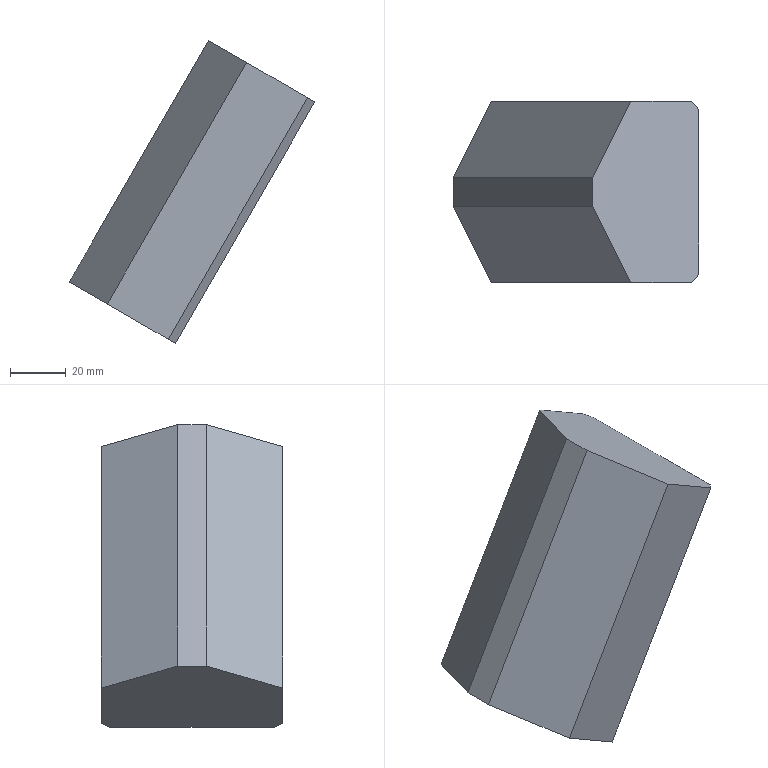Part | NX | features solid 2 | 1 solid | 10 faces | box 88.105 x 65 x 108.603 mm | volume 242059 mm3 | plane 10
STEP:
#1=CARTESIAN_POINT('',(295.929,67.5,17.1));
#2=VERTEX_POINT('',#1);
#3=CARTESIAN_POINT('',(317.784,67.5,4.482));
#4=VERTEX_POINT('',#3);
#5=CARTESIAN_POINT('',(279.679,67.5,26.482));
#6=DIRECTION('',(0.866,0.,-0.5));
#7=VECTOR('',#6,1000.);
#8=LINE('',#5,#7);
#9=EDGE_CURVE('',#2,#4,#8,.T.);
#10=ORIENTED_EDGE('',*,*,#9,.F.);
#11=CARTESIAN_POINT('',(245.929,67.5,-69.502));
#12=VERTEX_POINT('',#11);
#13=CARTESIAN_POINT('',(308.429,67.5,38.751));
#14=DIRECTION('',(0.5,0.,0.866));
#15=VECTOR('',#14,1000.);
#16=LINE('',#13,#15);
#17=EDGE_CURVE('',#12,#2,#16,.T.);
#18=ORIENTED_EDGE('',*,*,#17,.F.);
#19=CARTESIAN_POINT('',(267.784,67.5,-82.12));
#20=VERTEX_POINT('',#19);
#21=CARTESIAN_POINT('',(229.679,67.5,-60.12));
#22=DIRECTION('',(0.866,0.,-0.5));
#23=VECTOR('',#22,1000.);
#24=LINE('',#21,#23);
#25=EDGE_CURVE('',#12,#20,#24,.T.);
#26=ORIENTED_EDGE('',*,*,#25,.T.);
#27=CARTESIAN_POINT('',(330.284,67.5,26.133));
#28=DIRECTION('',(-0.5,0.,-0.866));
#29=VECTOR('',#28,1000.);
#30=LINE('',#27,#29);
#31=EDGE_CURVE('',#4,#20,#30,.T.);
#32=ORIENTED_EDGE('',*,*,#31,.F.);
#33=EDGE_LOOP('',(#10,#18,#26,#32));
#34=FACE_BOUND('',#33,.T.);
#35=CARTESIAN_POINT('',(292.179,67.5,48.133));
#36=DIRECTION('',(0.,-1.,0.));
#37=DIRECTION('',(0.866,0.,-0.5));
#38=AXIS2_PLACEMENT_3D('',#35,#36,#37);
#39=PLANE('',#38);
#40=ADVANCED_FACE('',(#34),#39,.T.);
#41=ORIENTED_EDGE('',*,*,#25,.F.);
#42=CARTESIAN_POINT('',(232.277,94.804,-61.62));
#43=VERTEX_POINT('',#42);
#44=CARTESIAN_POINT('',(217.491,124.375,-53.084));
#45=DIRECTION('',(0.433,-0.866,-0.25));
#46=VECTOR('',#45,1000.);
#47=LINE('',#44,#46);
#48=EDGE_CURVE('',#43,#12,#47,.T.);
#49=ORIENTED_EDGE('',*,*,#48,.F.);
#50=CARTESIAN_POINT('',(232.277,105.196,-61.62));
#51=VERTEX_POINT('',#50);
#52=CARTESIAN_POINT('',(232.277,132.5,-61.62));
#53=DIRECTION('',(0.,1.,0.));
#54=VECTOR('',#53,1000.);
#55=LINE('',#52,#54);
#56=EDGE_CURVE('',#43,#51,#55,.T.);
#57=ORIENTED_EDGE('',*,*,#56,.T.);
#58=CARTESIAN_POINT('',(245.929,132.5,-69.502));
#59=VERTEX_POINT('',#58);
#60=CARTESIAN_POINT('',(241.866,124.375,-67.157));
#61=DIRECTION('',(0.433,0.866,-0.25));
#62=VECTOR('',#61,1000.);
#63=LINE('',#60,#62);
#64=EDGE_CURVE('',#51,#59,#63,.T.);
#65=ORIENTED_EDGE('',*,*,#64,.T.);
#66=CARTESIAN_POINT('',(267.784,132.5,-82.12));
#67=VERTEX_POINT('',#66);
#68=CARTESIAN_POINT('',(229.679,132.5,-60.12));
#69=DIRECTION('',(-0.866,0.,0.5));
#70=VECTOR('',#69,1000.);
#71=LINE('',#68,#70);
#72=EDGE_CURVE('',#59,#67,#71,.F.);
#73=ORIENTED_EDGE('',*,*,#72,.T.);
#74=CARTESIAN_POINT('',(270.382,129.5,-83.62));
#75=VERTEX_POINT('',#74);
#76=CARTESIAN_POINT('',(248.731,154.5,-71.12));
#77=DIRECTION('',(0.6124,-0.7071,-0.3536));
#78=VECTOR('',#77,1000.);
#79=LINE('',#76,#78);
#80=EDGE_CURVE('',#75,#67,#79,.F.);
#81=ORIENTED_EDGE('',*,*,#80,.F.);
#82=CARTESIAN_POINT('',(270.382,70.5,-83.62));
#83=VERTEX_POINT('',#82);
#84=CARTESIAN_POINT('',(270.382,132.5,-83.62));
#85=DIRECTION('',(0.,1.,0.));
#86=VECTOR('',#85,1000.);
#87=LINE('',#84,#86);
#88=EDGE_CURVE('',#75,#83,#87,.F.);
#89=ORIENTED_EDGE('',*,*,#88,.T.);
#90=CARTESIAN_POINT('',(276.877,78.,-87.37));
#91=DIRECTION('',(0.6124,0.7071,-0.3536));
#92=VECTOR('',#91,1000.);
#93=LINE('',#90,#92);
#94=EDGE_CURVE('',#20,#83,#93,.T.);
#95=ORIENTED_EDGE('',*,*,#94,.F.);
#96=EDGE_LOOP('',(#41,#49,#57,#65,#73,#81,#89,#95));
#97=FACE_BOUND('',#96,.T.);
#98=CARTESIAN_POINT('',(229.679,132.5,-60.12));
#99=DIRECTION('',(-0.5,0.,-0.866));
#100=DIRECTION('',(0.866,0.,-0.5));
#101=AXIS2_PLACEMENT_3D('',#98,#99,#100);
#102=PLANE('',#101);
#103=ADVANCED_FACE('',(#97),#102,.T.);
#104=CARTESIAN_POINT('',(320.382,129.5,2.982));
#105=VERTEX_POINT('',#104);
#106=CARTESIAN_POINT('',(320.382,70.5,2.982));
#107=VERTEX_POINT('',#106);
#108=CARTESIAN_POINT('',(320.382,132.5,2.982));
#109=DIRECTION('',(0.,1.,0.));
#110=VECTOR('',#109,1000.);
#111=LINE('',#108,#110);
#112=EDGE_CURVE('',#105,#107,#111,.F.);
#113=ORIENTED_EDGE('',*,*,#112,.F.);
#114=CARTESIAN_POINT('',(317.784,132.5,4.482));
#115=VERTEX_POINT('',#114);
#116=CARTESIAN_POINT('',(320.382,129.5,2.982));
#117=DIRECTION('',(-0.6124,0.7071,0.3536));
#118=VECTOR('',#117,1000.);
#119=LINE('',#116,#118);
#120=EDGE_CURVE('',#115,#105,#119,.F.);
#121=ORIENTED_EDGE('',*,*,#120,.F.);
#122=CARTESIAN_POINT('',(295.929,132.5,17.1));
#123=VERTEX_POINT('',#122);
#124=CARTESIAN_POINT('',(279.679,132.5,26.482));
#125=DIRECTION('',(-0.866,0.,0.5));
#126=VECTOR('',#125,1000.);
#127=LINE('',#124,#126);
#128=EDGE_CURVE('',#123,#115,#127,.F.);
#129=ORIENTED_EDGE('',*,*,#128,.F.);
#130=CARTESIAN_POINT('',(282.277,105.196,24.982));
#131=VERTEX_POINT('',#130);
#132=CARTESIAN_POINT('',(291.866,124.375,19.446));
#133=DIRECTION('',(0.433,0.866,-0.25));
#134=VECTOR('',#133,1000.);
#135=LINE('',#132,#134);
#136=EDGE_CURVE('',#131,#123,#135,.T.);
#137=ORIENTED_EDGE('',*,*,#136,.F.);
#138=CARTESIAN_POINT('',(282.277,94.804,24.982));
#139=VERTEX_POINT('',#138);
#140=CARTESIAN_POINT('',(282.277,132.5,24.982));
#141=DIRECTION('',(0.,1.,0.));
#142=VECTOR('',#141,1000.);
#143=LINE('',#140,#142);
#144=EDGE_CURVE('',#139,#131,#143,.T.);
#145=ORIENTED_EDGE('',*,*,#144,.F.);
#146=CARTESIAN_POINT('',(267.491,124.375,33.519));
#147=DIRECTION('',(0.433,-0.866,-0.25));
#148=VECTOR('',#147,1000.);
#149=LINE('',#146,#148);
#150=EDGE_CURVE('',#139,#2,#149,.T.);
#151=ORIENTED_EDGE('',*,*,#150,.T.);
#152=ORIENTED_EDGE('',*,*,#9,.T.);
#153=CARTESIAN_POINT('',(317.784,67.5,4.482));
#154=DIRECTION('',(-0.6124,-0.7071,0.3536));
#155=VECTOR('',#154,1000.);
#156=LINE('',#153,#155);
#157=EDGE_CURVE('',#107,#4,#156,.T.);
#158=ORIENTED_EDGE('',*,*,#157,.F.);
#159=EDGE_LOOP('',(#113,#121,#129,#137,#145,#151,#152,#158));
#160=FACE_BOUND('',#159,.T.);
#161=CARTESIAN_POINT('',(279.679,132.5,26.482));
#162=DIRECTION('',(-0.5,0.,-0.866));
#163=DIRECTION('',(0.866,0.,-0.5));
#164=AXIS2_PLACEMENT_3D('',#161,#162,#163);
#165=PLANE('',#164);
#166=ADVANCED_FACE('',(#160),#165,.F.);
#167=ORIENTED_EDGE('',*,*,#88,.F.);
#168=CARTESIAN_POINT('',(332.882,129.5,24.633));
#169=DIRECTION('',(0.5,0.,0.866));
#170=VECTOR('',#169,1000.);
#171=LINE('',#168,#170);
#172=EDGE_CURVE('',#105,#75,#171,.F.);
#173=ORIENTED_EDGE('',*,*,#172,.F.);
#174=ORIENTED_EDGE('',*,*,#112,.T.);
#175=CARTESIAN_POINT('',(332.882,70.5,24.633));
#176=DIRECTION('',(-0.5,0.,-0.866));
#177=VECTOR('',#176,1000.);
#178=LINE('',#175,#177);
#179=EDGE_CURVE('',#83,#107,#178,.F.);
#180=ORIENTED_EDGE('',*,*,#179,.F.);
#181=EDGE_LOOP('',(#167,#173,#174,#180));
#182=FACE_BOUND('',#181,.T.);
#183=CARTESIAN_POINT('',(332.882,132.5,24.633));
#184=DIRECTION('',(-0.866,0.,0.5));
#185=DIRECTION('',(0.,-1.,0.));
#186=AXIS2_PLACEMENT_3D('',#183,#184,#185);
#187=PLANE('',#186);
#188=ADVANCED_FACE('',(#182),#187,.F.);
#189=ORIENTED_EDGE('',*,*,#72,.F.);
#190=CARTESIAN_POINT('',(308.429,132.5,38.751));
#191=DIRECTION('',(-0.5,0.,-0.866));
#192=VECTOR('',#191,1000.);
#193=LINE('',#190,#192);
#194=EDGE_CURVE('',#59,#123,#193,.F.);
#195=ORIENTED_EDGE('',*,*,#194,.T.);
#196=ORIENTED_EDGE('',*,*,#128,.T.);
#197=CARTESIAN_POINT('',(330.284,132.5,26.133));
#198=DIRECTION('',(-0.5,0.,-0.866));
#199=VECTOR('',#198,1000.);
#200=LINE('',#197,#199);
#201=EDGE_CURVE('',#67,#115,#200,.F.);
#202=ORIENTED_EDGE('',*,*,#201,.F.);
#203=EDGE_LOOP('',(#189,#195,#196,#202));
#204=FACE_BOUND('',#203,.T.);
#205=CARTESIAN_POINT('',(292.179,132.5,48.133));
#206=DIRECTION('',(0.,-1.,0.));
#207=DIRECTION('',(0.866,0.,-0.5));
#208=AXIS2_PLACEMENT_3D('',#205,#206,#207);
#209=PLANE('',#208);
#210=ADVANCED_FACE('',(#204),#209,.F.);
#211=CARTESIAN_POINT('',(294.777,94.804,46.633));
#212=DIRECTION('',(-0.5,0.,-0.866));
#213=VECTOR('',#212,1000.);
#214=LINE('',#211,#213);
#215=EDGE_CURVE('',#139,#43,#214,.T.);
#216=ORIENTED_EDGE('',*,*,#215,.T.);
#217=ORIENTED_EDGE('',*,*,#48,.T.);
#218=ORIENTED_EDGE('',*,*,#17,.T.);
#219=ORIENTED_EDGE('',*,*,#150,.F.);
#220=EDGE_LOOP('',(#216,#217,#218,#219));
#221=FACE_BOUND('',#220,.T.);
#222=CARTESIAN_POINT('',(292.179,100.,48.133));
#223=DIRECTION('',(-0.75,-0.5,0.433));
#224=DIRECTION('',(0.433,-0.866,-0.25));
#225=AXIS2_PLACEMENT_3D('',#222,#223,#224);
#226=PLANE('',#225);
#227=ADVANCED_FACE('',(#221),#226,.T.);
#228=ORIENTED_EDGE('',*,*,#136,.T.);
#229=ORIENTED_EDGE('',*,*,#194,.F.);
#230=ORIENTED_EDGE('',*,*,#64,.F.);
#231=CARTESIAN_POINT('',(294.777,105.196,46.633));
#232=DIRECTION('',(-0.5,0.,-0.866));
#233=VECTOR('',#232,1000.);
#234=LINE('',#231,#233);
#235=EDGE_CURVE('',#131,#51,#234,.T.);
#236=ORIENTED_EDGE('',*,*,#235,.F.);
#237=EDGE_LOOP('',(#228,#229,#230,#236));
#238=FACE_BOUND('',#237,.T.);
#239=CARTESIAN_POINT('',(292.179,100.,48.133));
#240=DIRECTION('',(0.75,-0.5,-0.433));
#241=DIRECTION('',(0.433,0.866,-0.25));
#242=AXIS2_PLACEMENT_3D('',#239,#240,#241);
#243=PLANE('',#242);
#244=ADVANCED_FACE('',(#238),#243,.F.);
#245=ORIENTED_EDGE('',*,*,#215,.F.);
#246=ORIENTED_EDGE('',*,*,#144,.T.);
#247=ORIENTED_EDGE('',*,*,#235,.T.);
#248=ORIENTED_EDGE('',*,*,#56,.F.);
#249=EDGE_LOOP('',(#245,#246,#247,#248));
#250=FACE_BOUND('',#249,.T.);
#251=CARTESIAN_POINT('',(257.277,100.,-18.319));
#252=DIRECTION('',(0.866,0.,-0.5));
#253=DIRECTION('',(0.5,0.,0.866));
#254=AXIS2_PLACEMENT_3D('',#251,#252,#253);
#255=PLANE('',#254);
#256=ADVANCED_FACE('',(#250),#255,.F.);
#257=ORIENTED_EDGE('',*,*,#157,.T.);
#258=ORIENTED_EDGE('',*,*,#31,.T.);
#259=ORIENTED_EDGE('',*,*,#94,.T.);
#260=ORIENTED_EDGE('',*,*,#179,.T.);
#261=EDGE_LOOP('',(#257,#258,#259,#260));
#262=FACE_BOUND('',#261,.T.);
#263=CARTESIAN_POINT('',(330.284,67.5,26.133));
#264=DIRECTION('',(0.6124,-0.7071,-0.3536));
#265=DIRECTION('',(0.6124,0.7071,-0.3536));
#266=AXIS2_PLACEMENT_3D('',#263,#264,#265);
#267=PLANE('',#266);
#268=ADVANCED_FACE('',(#262),#267,.T.);
#269=ORIENTED_EDGE('',*,*,#120,.T.);
#270=ORIENTED_EDGE('',*,*,#172,.T.);
#271=ORIENTED_EDGE('',*,*,#80,.T.);
#272=ORIENTED_EDGE('',*,*,#201,.T.);
#273=EDGE_LOOP('',(#269,#270,#271,#272));
#274=FACE_BOUND('',#273,.T.);
#275=CARTESIAN_POINT('',(332.882,129.5,24.633));
#276=DIRECTION('',(-0.6124,-0.7071,0.3536));
#277=DIRECTION('',(0.6124,-0.7071,-0.3536));
#278=AXIS2_PLACEMENT_3D('',#275,#276,#277);
#279=PLANE('',#278);
#280=ADVANCED_FACE('',(#274),#279,.F.);
#281=CLOSED_SHELL('',(#40,#103,#166,#188,#210,#227,#244,#256,#268,#280));
#282=MANIFOLD_SOLID_BREP('',#281);
#283=(LENGTH_UNIT()NAMED_UNIT(*)SI_UNIT(.MILLI.,.METRE.));
#284=UNCERTAINTY_MEASURE_WITH_UNIT(LENGTH_MEASURE(0.00001),#283,'','');
#285=(NAMED_UNIT(*)PLANE_ANGLE_UNIT()SI_UNIT($,.RADIAN.));
#286=(NAMED_UNIT(*)SI_UNIT($,.STERADIAN.)SOLID_ANGLE_UNIT());
#287=(GEOMETRIC_REPRESENTATION_CONTEXT(3)GLOBAL_UNCERTAINTY_ASSIGNED_CONTEXT((#284))GLOBAL_UNIT_ASSIGNED_CONTEXT((#283,#285,#286))REPRESENTATION_CONTEXT('',''));
#288=ADVANCED_BREP_SHAPE_REPRESENTATION('',(#282),#287);